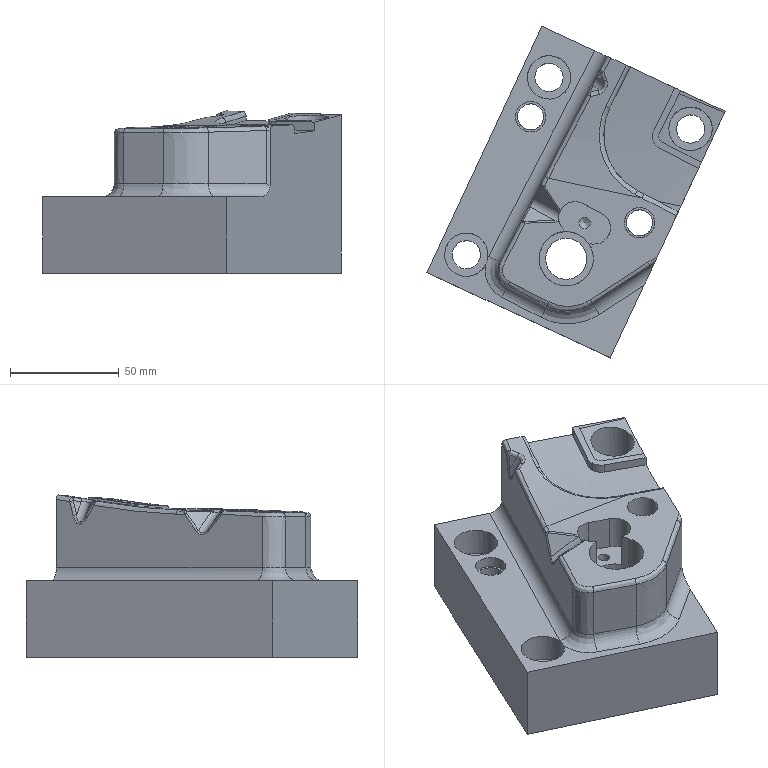Part | STEP file | gslz 2016.10.28-13_id254_x_t | 1 solid | 95 faces | box 137.114 x 152.592 x 74.542 mm | volume 551443 mm3 | spline 36 | plane 25 | cylinder 24 | other 7 | sphere 2 | cone 1 | commonest cylinder face diameters 12 x5 13 x3 20 x3 2 x2 4 x2 6.5 x2